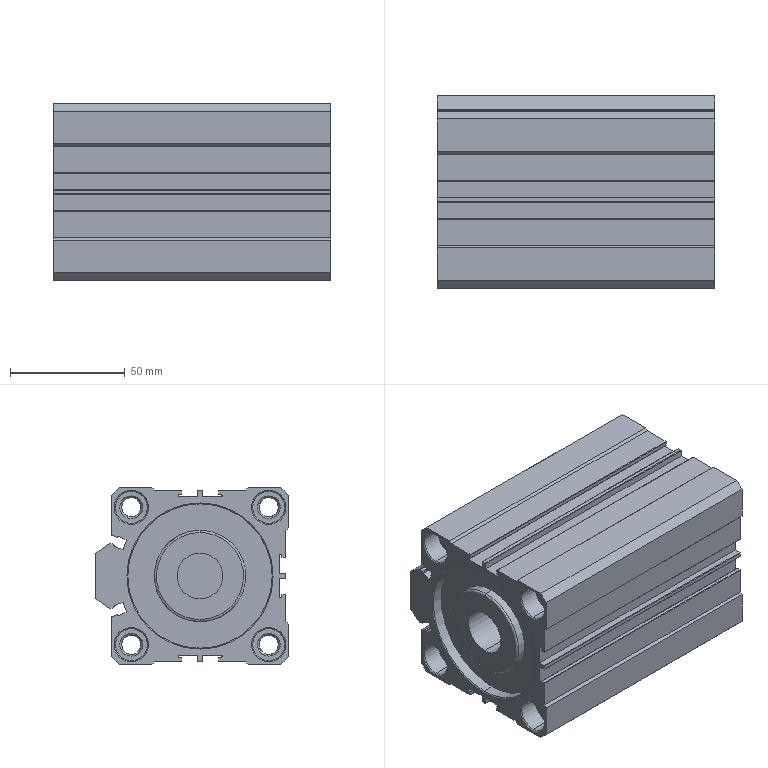Part | SolidWorks | features BaseBody 1 | 1 solid | 227 faces | box 121 x 84 x 77 mm | volume 331799 mm3 | cylinder 92 | plane 89 | cone 44 | spline 2 | commonest cylinder face diameters 0.4 x35 14 x16 0.8 x15 8.376 x8 63 x6 11.445 x4